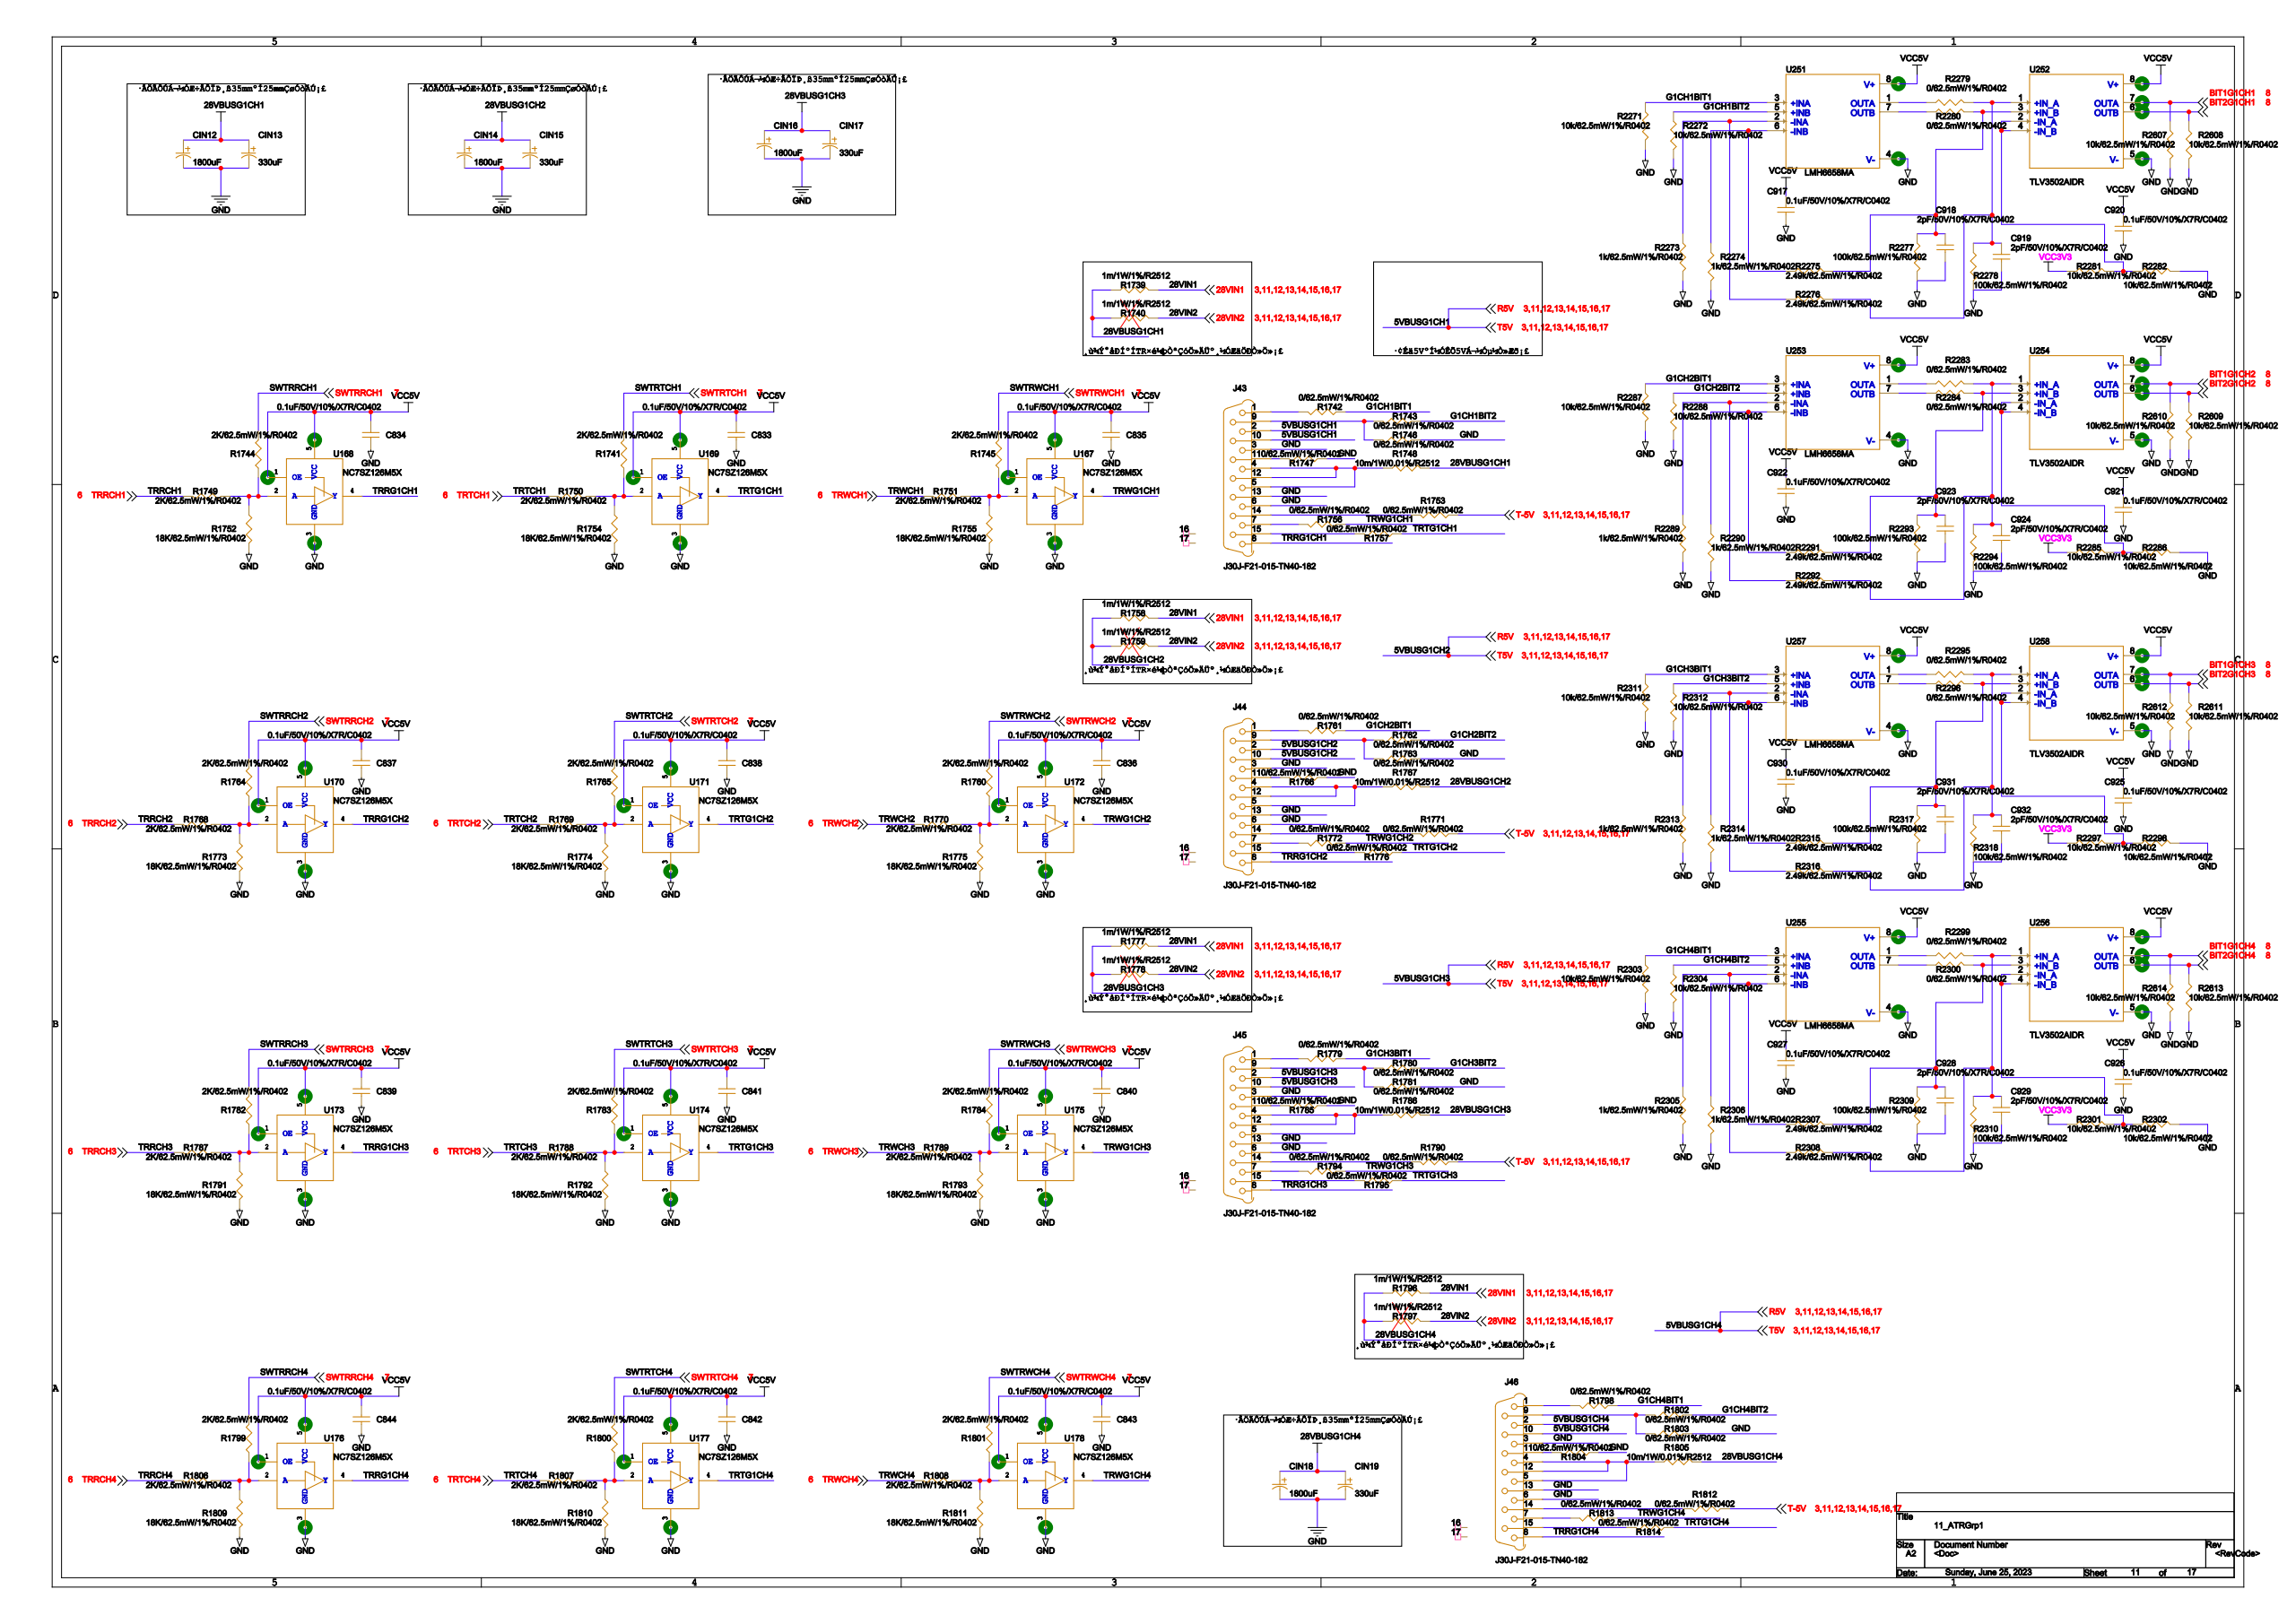Circuit board | Cadence Allegro | 1997 parts | 1536 nets | one sheet of the schematic
Parts on this sheet (reference | value | footprint):
C833 | 0.1uF/50V/10%/X7R/C0402 | 0402
C834 | 0.1uF/50V/10%/X7R/C0402 | 0402
C835 | 0.1uF/50V/10%/X7R/C0402 | 0402
C836 | 0.1uF/50V/10%/X7R/C0402 | 0402
C837 | 0.1uF/50V/10%/X7R/C0402 | 0402
C838 | 0.1uF/50V/10%/X7R/C0402 | 0402
C839 | 0.1uF/50V/10%/X7R/C0402 | 0402
C840 | 0.1uF/50V/10%/X7R/C0402 | 0402
C841 | 0.1uF/50V/10%/X7R/C0402 | 0402
C842 | 0.1uF/50V/10%/X7R/C0402 | 0402
C843 | 0.1uF/50V/10%/X7R/C0402 | 0402
C844 | 0.1uF/50V/10%/X7R/C0402 | 0402
C918 | 2pF/50V/10%/X7R/C0402 | 0402
C919 | 2pF/50V/10%/X7R/C0402 | 0402
C920 | 0.1uF/50V/10%/X7R/C0402 | 0402
C921 | 0.1uF/50V/10%/X7R/C0402 | 0402
C923 | 2pF/50V/10%/X7R/C0402 | 0402
C924 | 2pF/50V/10%/X7R/C0402 | 0402
C925 | 0.1uF/50V/10%/X7R/C0402 | 0402
C926 | 0.1uF/50V/10%/X7R/C0402 | 0402
C928 | 2pF/50V/10%/X7R/C0402 | 0402
C929 | 2pF/50V/10%/X7R/C0402 | 0402
C931 | 2pF/50V/10%/X7R/C0402 | 0402
C932 | 2pF/50V/10%/X7R/C0402 | 0402
CIN12 | ECF1HM182M27OTPO | AP-SMD_BD18-L27-W6_6-LS7_21
CIN13 | ECF1JM331G20OTPO | AP-SMD_BD10-L20-W6_6-LS7_21
CIN14 | ECF1HM182M27OTPO | AP-SMD_BD18-L27-W6_6-LS7_21
CIN15 | ECF1JM331G20OTPO | AP-SMD_BD10-L20-W6_6-LS7_21
CIN16 | ECF1HM182M27OTPO | AP-SMD_BD18-L27-W6_6-LS7_21
CIN17 | ECF1JM331G20OTPO | AP-SMD_BD10-L20-W6_6-LS7_21
CIN18 | ECF1HM182M27OTPO | AP-SMD_BD18-L27-W6_6-LS7_21
CIN19 | ECF1JM331G20OTPO | AP-SMD_BD10-L20-W6_6-LS7_21
J43 | J30J-F21-015-TN40-182 | J30J-F21-015-TN40-182
J44 | J30J-F21-015-TN40-182 | J30J-F21-015-TN40-182
J45 | J30J-F21-015-TN40-182 | J30J-F21-015-TN40-182
J46 | J30J-F21-015-TN40-182 | J30J-F21-015-TN40-182
R1739 | 1m/1W/1%/R2512 | 2512
R1740 | 1m/1W/1%/R2512 | 2512
R1741 | 2K/62.5mW/1%/R0402 | 0402
R1742 | 0/62.5mW/1%/R0402 | 0402
R1743 | 0/62.5mW/1%/R0402 | 0402
R1744 | 2K/62.5mW/1%/R0402 | 0402
R1745 | 2K/62.5mW/1%/R0402 | 0402
R1746 | 0/62.5mW/1%/R0402 | 0402
R1747 | 0/62.5mW/1%/R0402 | 0402
R1748 | 10m/1W/0.01%/R2512 | 2512
R1749 | 2K/62.5mW/1%/R0402 | 0402
R1750 | 2K/62.5mW/1%/R0402 | 0402
R1751 | 2K/62.5mW/1%/R0402 | 0402
R1752 | 18K/62.5mW/1%/R0402 | 0402
R1753 | 0/62.5mW/1%/R0402 | 0402
R1754 | 18K/62.5mW/1%/R0402 | 0402
R1755 | 18K/62.5mW/1%/R0402 | 0402
R1756 | 0/62.5mW/1%/R0402 | 0402
R1757 | 0/62.5mW/1%/R0402 | 0402
R1758 | 1m/1W/1%/R2512 | 2512
R1759 | 1m/1W/1%/R2512 | 2512
R1760 | 2K/62.5mW/1%/R0402 | 0402
R1761 | 0/62.5mW/1%/R0402 | 0402
R1762 | 0/62.5mW/1%/R0402 | 0402
R1763 | 0/62.5mW/1%/R0402 | 0402
R1764 | 2K/62.5mW/1%/R0402 | 0402
R1765 | 2K/62.5mW/1%/R0402 | 0402
R1766 | 0/62.5mW/1%/R0402 | 0402
R1767 | 10m/1W/0.01%/R2512 | 2512
R1768 | 2K/62.5mW/1%/R0402 | 0402
R1769 | 2K/62.5mW/1%/R0402 | 0402
R1770 | 2K/62.5mW/1%/R0402 | 0402
R1771 | 0/62.5mW/1%/R0402 | 0402
R1772 | 0/62.5mW/1%/R0402 | 0402
R1773 | 18K/62.5mW/1%/R0402 | 0402
R1774 | 18K/62.5mW/1%/R0402 | 0402
R1775 | 18K/62.5mW/1%/R0402 | 0402
R1776 | 0/62.5mW/1%/R0402 | 0402
R1777 | 1m/1W/1%/R2512 | 2512
R1778 | 1m/1W/1%/R2512 | 2512
R1779 | 0/62.5mW/1%/R0402 | 0402
R1780 | 0/62.5mW/1%/R0402 | 0402
R1781 | 0/62.5mW/1%/R0402 | 0402
R1782 | 2K/62.5mW/1%/R0402 | 0402
R1783 | 2K/62.5mW/1%/R0402 | 0402
R1784 | 2K/62.5mW/1%/R0402 | 0402
R1785 | 0/62.5mW/1%/R0402 | 0402
R1786 | 10m/1W/0.01%/R2512 | 2512
R1787 | 2K/62.5mW/1%/R0402 | 0402
R1788 | 2K/62.5mW/1%/R0402 | 0402
R1789 | 2K/62.5mW/1%/R0402 | 0402
R1790 | 0/62.5mW/1%/R0402 | 0402
R1791 | 18K/62.5mW/1%/R0402 | 0402
R1792 | 18K/62.5mW/1%/R0402 | 0402
R1793 | 18K/62.5mW/1%/R0402 | 0402
R1794 | 0/62.5mW/1%/R0402 | 0402
R1795 | 0/62.5mW/1%/R0402 | 0402
R1796 | 1m/1W/1%/R2512 | 2512
R1797 | 1m/1W/1%/R2512 | 2512
R1798 | 0/62.5mW/1%/R0402 | 0402
R1799 | 2K/62.5mW/1%/R0402 | 0402
R1800 | 2K/62.5mW/1%/R0402 | 0402
R1801 | 2K/62.5mW/1%/R0402 | 0402
R1802 | 0/62.5mW/1%/R0402 | 0402
R1803 | 0/62.5mW/1%/R0402 | 0402
R1804 | 0/62.5mW/1%/R0402 | 0402
R1805 | 10m/1W/0.01%/R2512 | 2512
R1806 | 2K/62.5mW/1%/R0402 | 0402
R1807 | 2K/62.5mW/1%/R0402 | 0402
R1808 | 2K/62.5mW/1%/R0402 | 0402
R1809 | 18K/62.5mW/1%/R0402 | 0402
R1810 | 18K/62.5mW/1%/R0402 | 0402
R1811 | 18K/62.5mW/1%/R0402 | 0402
R1812 | 0/62.5mW/1%/R0402 | 0402
R1813 | 0/62.5mW/1%/R0402 | 0402
R1814 | 0/62.5mW/1%/R0402 | 0402
R2271 | 10k/62.5mW/1%/R0402 | 0402
R2272 | 10k/62.5mW/1%/R0402 | 0402
R2273 | 1K/62.5mW/1%/R0402 | 0402
R2274 | 1K/62.5mW/1%/R0402 | 0402
R2276 | 2.49k/62.5mW/1%/R0402 | 0402
R2277 | 100k/62.5mW/1%/R0402 | 0402
R2278 | 100k/62.5mW/1%/R0402 | 0402
R2279 | 0/62.5mW/1%/R0402 | 0402
R2280 | 0/62.5mW/1%/R0402 | 0402
R2281 | 10k/62.5mW/1%/R0402 | 0402
R2282 | 10k/62.5mW/1%/R0402 | 0402
R2283 | 0/62.5mW/1%/R0402 | 0402
R2284 | 0/62.5mW/1%/R0402 | 0402
R2285 | 10k/62.5mW/1%/R0402 | 0402
R2286 | 10k/62.5mW/1%/R0402 | 0402
R2287 | 10k/62.5mW/1%/R0402 | 0402
R2288 | 10k/62.5mW/1%/R0402 | 0402
R2289 | 1K/62.5mW/1%/R0402 | 0402
R2290 | 1K/62.5mW/1%/R0402 | 0402
R2292 | 2.49k/62.5mW/1%/R0402 | 0402
R2293 | 100k/62.5mW/1%/R0402 | 0402
R2294 | 100k/62.5mW/1%/R0402 | 0402
R2295 | 0/62.5mW/1%/R0402 | 0402
R2296 | 0/62.5mW/1%/R0402 | 0402
R2297 | 10k/62.5mW/1%/R0402 | 0402
R2298 | 10k/62.5mW/1%/R0402 | 0402
R2299 | 0/62.5mW/1%/R0402 | 0402
R2300 | 0/62.5mW/1%/R0402 | 0402
R2301 | 10k/62.5mW/1%/R0402 | 0402
R2302 | 10k/62.5mW/1%/R0402 | 0402
R2303 | 10k/62.5mW/1%/R0402 | 0402
R2304 | 10k/62.5mW/1%/R0402 | 0402
R2305 | 1K/62.5mW/1%/R0402 | 0402
R2306 | 1K/62.5mW/1%/R0402 | 0402
R2308 | 2.49k/62.5mW/1%/R0402 | 0402
R2309 | 100k/62.5mW/1%/R0402 | 0402
R2310 | 100k/62.5mW/1%/R0402 | 0402
R2311 | 10k/62.5mW/1%/R0402 | 0402
R2312 | 10k/62.5mW/1%/R0402 | 0402
R2313 | 1K/62.5mW/1%/R0402 | 0402
R2314 | 1K/62.5mW/1%/R0402 | 0402
R2316 | 2.49k/62.5mW/1%/R0402 | 0402
R2317 | 100k/62.5mW/1%/R0402 | 0402
R2318 | 100k/62.5mW/1%/R0402 | 0402
R2607 | 10k/62.5mW/1%/R0402 | 0402
R2608 | 10k/62.5mW/1%/R0402 | 0402
R2609 | 10k/62.5mW/1%/R0402 | 0402
R2610 | 10k/62.5mW/1%/R0402 | 0402
R2611 | 10k/62.5mW/1%/R0402 | 0402
R2612 | 10k/62.5mW/1%/R0402 | 0402
R2613 | 10k/62.5mW/1%/R0402 | 0402
R2614 | 10k/62.5mW/1%/R0402 | 0402
U167 | NC7SZ126M5X | SOT-23-5
U168 | NC7SZ126M5X | SOT-23-5
U169 | NC7SZ126M5X | SOT-23-5
U170 | NC7SZ126M5X | SOT-23-5
U171 | NC7SZ126M5X | SOT-23-5
U172 | NC7SZ126M5X | SOT-23-5
U173 | NC7SZ126M5X | SOT-23-5
U174 | NC7SZ126M5X | SOT-23-5
U175 | NC7SZ126M5X | SOT-23-5
U176 | NC7SZ126M5X | SOT-23-5
U177 | NC7SZ126M5X | SOT-23-5
U178 | NC7SZ126M5X | SOT-23-5
U251 | LMH6658MA | SOIC127P599X175-8N
U253 | LMH6658MA | SOIC127P599X175-8N
U255 | LMH6658MA | SOIC127P599X175-8N
U257 | LMH6658MA | SOIC127P599X175-8N
Nets of these parts (net: part-pin ...):
3.3V: R2281-1 R2285-1 R2297-1 R2301-1
AGND: C833-2 C834-2 C835-2 C836-2 C837-2 C838-2 C839-2 C840-2 C841-2 C842-2 C843-2 C844-2 C918-2 C919-2 C920-2 C921-2 C923-2 C924-2 C925-2 C926-2 C928-2 C929-2 C931-2 C932-2 CIN12-2 CIN13-2 CIN14-2 CIN15-2 CIN16-2 CIN17-2 CIN18-2 CIN19-2 J43-3 J43-6 J43-13 J44-3 J44-6 J44-13 J45-3 J45-6 J45-13 J46-3 J46-6 J46-13 R1746-1 R1747-1 R1752-1 R1754-1 R1755-1 R1763-1 R1766-1 R1773-1 R1774-1 R1775-1 R1781-1 R1785-1 R1791-1 R1792-1 R1793-1 R1803-1 R1804-1 R1809-1 R1810-1 R1811-1 R2271-2 R2272-2 R2273-2 R2274-2 R2277-2 R2278-2 R2282-2 R2286-2 R2287-2 R2288-2 R2289-2 R2290-2 R2293-2 R2294-2 R2298-2 R2302-2 R2303-2 R2304-2 R2305-2 R2306-2 R2309-2 R2310-2 R2311-2 R2312-2 R2313-2 R2314-2 R2317-2 R2318-2 R2607-2 R2608-2 R2609-2 R2610-2 R2611-2 R2612-2 R2613-2 R2614-2 U167-3 U168-3 U169-3 U170-3 U171-3 U172-3 U173-3 U174-3 U175-3 U176-3 U177-3 U178-3 U251-4 U253-4 U255-4 U257-4
VCC5V: C833-1 C834-1 C835-1 C836-1 C837-1 C838-1 C839-1 C840-1 C841-1 C842-1 C843-1 C844-1 C920-1 C921-1 C925-1 C926-1 U167-1 U167-5 U168-1 U168-5 U169-1 U169-5 U170-1 U170-5 U171-1 U171-5 U172-1 U172-5 U173-1 U173-5 U174-1 U174-5 U175-1 U175-5 U176-1 U176-5 U177-1 U177-5 U178-1 U178-5 U251-8 U253-8 U255-8 U257-8
N24388183: R2274-1 U251-6
N24388197: C918-1 R2277-1 R2280-2
N24388176: R2273-1 R2276-1 U251-2
N24388194: C919-1 R2276-2 R2278-1 R2279-2
N24389507: R2290-1 U253-6
N24389517: C923-1 R2284-2 R2293-1
N24389503: R2289-1 R2292-1 U253-2
N24389515: C924-1 R2283-2 R2292-2 R2294-1
N24391507: R2306-1 U255-6
N24391517: C928-1 R2300-2 R2309-1
N24391495: R2305-1 R2308-1 U255-2
N24391515: C929-1 R2299-2 R2308-2 R2310-1
N24391327: R2314-1 U257-6
N24391337: C931-1 R2296-2 R2317-1
N24391323: R2313-1 R2316-1 U257-2
N24391335: C932-1 R2295-2 R2316-2 R2318-1
G1CH1BIT1: R1742-1 R2271-1 U251-3
G1CH1BIT2: R1743-1 R2272-1 U251-5
N24388188: R2279-1 U251-1
N24388191: R2280-1 U251-7
G1CH2BIT1: R1761-1 R2287-1 U253-3
G1CH2BIT2: R1762-1 R2288-1 U253-5
N24389511: R2283-1 U253-1
N24389513: R2284-1 U253-7
G1CH4BIT1: R1798-1 R2303-1 U255-3
G1CH4BIT2: R1802-1 R2304-1 U255-5
N24391511: R2299-1 U255-1
N24391513: R2300-1 U255-7
G1CH3BIT1: R1779-1 R2311-1 U257-3
G1CH3BIT2: R1780-1 R2312-1 U257-5
N24391331: R2295-1 U257-1
N24391333: R2296-1 U257-7
N24388509: R2281-2 R2282-1
BIT1G1CH1: R2607-1
BIT2G1CH1: R2608-1
N24389569: R2285-2 R2286-1
BIT1G1CH2: R2610-1
BIT2G1CH2: R2609-1
N24391569: R2301-2 R2302-1
BIT1G1CH4: R2614-1
BIT2G1CH4: R2613-1
N24391389: R2297-2 R2298-1
BIT1G1CH3: R2612-1
BIT2G1CH3: R2611-1
N23704713: J43-1 R1742-2
R5V: J43-2 J43-10 J44-2 J44-10 J45-2 J45-10 J46-2 J46-10
N23704748: J43-11 R1747-2
N23704755: J43-4 J43-5 J43-12 R1748-1
N23704790: J43-14 R1753-2
N23704804: J43-15 R1757-2
N23704797: J43-7 R1756-2
TRRG1CH1: J43-8 U168-4
N23704720: J43-9 R1743-2 R1746-2
N23720843: J44-1 R1761-2
N23720856: J44-11 R1766-2
N23720858: J44-4 J44-5 J44-12 R1767-1
N23720870: J44-14 R1771-2
N23720874: J44-15 R1776-2
N23720872: J44-7 R1772-2
TRRG1CH2: J44-8 U170-4
N23720845: J44-9 R1762-2 R1763-2
N23721470: J45-1 R1779-2
N23721483: J45-11 R1785-2
N23721485: J45-4 J45-5 J45-12 R1786-1
N23721497: J45-14 R1790-2
N23721501: J45-15 R1795-2
N23721499: J45-7 R1794-2
TRRG1CH3: J45-8 U173-4
N23721472: J45-9 R1780-2 R1781-2
N23722102: J46-1 R1798-2
N23722115: J46-11 R1804-2
N23722117: J46-4 J46-5 J46-12 R1805-1
N23722129: J46-14 R1812-2
N23722133: J46-15 R1814-2
N23722131: J46-7 R1813-2
TRRG1CH4: J46-8 U176-4
N23722104: J46-9 R1802-2 R1803-2
28VIN1: R1739-2 R1758-2 R1777-2 R1796-2
T-5V: R1753-1 R1771-1 R1790-1 R1812-1
28VIN2: R1740-2 R1759-2 R1778-2 R1797-2
28VBUSG1CH1: CIN12-1 CIN13-1 R1739-1 R1740-1 R1748-2
28VBUSG1CH2: CIN14-1 CIN15-1 R1758-1 R1759-1 R1767-2
28VBUSG1CH3: CIN16-1 CIN17-1 R1777-1 R1778-1 R1786-2
28VBUSG1CH4: CIN18-1 CIN19-1 R1796-1 R1797-1 R1805-2
SWTRTCH1: R1741-1
N23998857: R1741-2 R1750-2 R1754-2 U169-2
SWTRRCH1: R1744-1
N23980235: R1744-2 R1749-2 R1752-2 U168-2
SWTRWCH1: R1745-1
N23999942: R1745-2 R1751-2 R1755-2 U167-2
TRRCH1: R1749-1
TRTCH1: R1750-1
TRWCH1: R1751-1
SWTRWCH2: R1760-1
N24000060: R1760-2 R1770-2 R1775-2 U172-2
SWTRRCH2: R1764-1
N23995239: R1764-2 R1768-2 R1773-2 U170-2
SWTRTCH2: R1765-1
N23998975: R1765-2 R1769-2 R1774-2 U171-2
TRRCH2: R1768-1
TRTCH2: R1769-1
TRWCH2: R1770-1
SWTRRCH3: R1782-1
N23995539: R1782-2 R1787-2 R1791-2 U173-2
SWTRTCH3: R1783-1
N23999101: R1783-2 R1788-2 R1792-2 U174-2
SWTRWCH3: R1784-1
N24000186: R1784-2 R1789-2 R1793-2 U175-2
TRRCH3: R1787-1
TRTCH3: R1788-1
TRWCH3: R1789-1
SWTRRCH4: R1799-1
N23995853: R1799-2 R1806-2 R1809-2 U176-2
SWTRTCH4: R1800-1
N23999219: R1800-2 R1807-2 R1810-2 U177-2
SWTRWCH4: R1801-1
N24000304: R1801-2 R1808-2 R1811-2 U178-2
TRRCH4: R1806-1
TRTCH4: R1807-1
TRWCH4: R1808-1
TRWG1CH1: R1756-1 U167-4
TRTG1CH1: R1757-1 U169-4
TRTG1CH2: R1776-1 U171-4
TRWG1CH2: R1772-1 U172-4
TRTG1CH3: R1795-1 U174-4
TRWG1CH3: R1794-1 U175-4
TRTG1CH4: R1814-1 U177-4
TRWG1CH4: R1813-1 U178-4